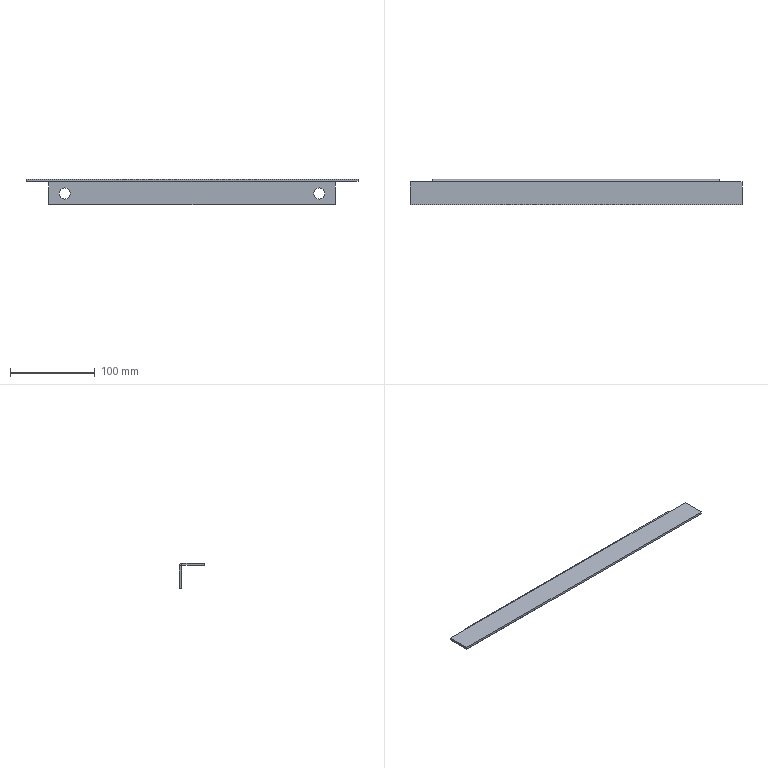Part | SolidWorks | features SMBaseFlange 2, Cut 1, EdgeFlange 1, FlatPattern 1, SheetMetal 1 | 1 solid | 20 faces | box 391 x 30 x 30 mm | volume 50792 mm3 | plane 14 | cylinder 6 | commonest cylinder face diameters 13 x4 1 x1 6 x1
STEP:
#1=CARTESIAN_POINT('',(150.,12.5,-23.25));
#2=VERTEX_POINT('',#1);
#3=CARTESIAN_POINT('',(150.,12.5,-10.25));
#4=VERTEX_POINT('',#3);
#5=CARTESIAN_POINT('',(150.,12.5,-16.75));
#6=DIRECTION('',(0.,1.,0.));
#7=DIRECTION('',(0.,0.,1.));
#8=AXIS2_PLACEMENT_3D('',#5,#6,#7);
#9=CIRCLE('',#8,6.5);
#10=EDGE_CURVE('',#2,#4,#9,.T.);
#11=ORIENTED_EDGE('',*,*,#10,.F.);
#12=CARTESIAN_POINT('',(150.,15.,-23.25));
#13=VERTEX_POINT('',#12);
#14=CARTESIAN_POINT('',(150.,12.5,-23.25));
#15=DIRECTION('',(0.,1.,0.));
#16=VECTOR('',#15,1000.);
#17=LINE('',#14,#16);
#18=EDGE_CURVE('',#2,#13,#17,.T.);
#19=ORIENTED_EDGE('',*,*,#18,.T.);
#20=CARTESIAN_POINT('',(150.,15.,-10.25));
#21=VERTEX_POINT('',#20);
#22=CARTESIAN_POINT('',(150.,15.,-16.75));
#23=DIRECTION('',(0.,1.,0.));
#24=DIRECTION('',(0.,0.,1.));
#25=AXIS2_PLACEMENT_3D('',#22,#23,#24);
#26=CIRCLE('',#25,6.5);
#27=EDGE_CURVE('',#13,#21,#26,.T.);
#28=ORIENTED_EDGE('',*,*,#27,.T.);
#29=CARTESIAN_POINT('',(150.,12.5,-10.25));
#30=DIRECTION('',(0.,1.,0.));
#31=VECTOR('',#30,1000.);
#32=LINE('',#29,#31);
#33=EDGE_CURVE('',#4,#21,#32,.T.);
#34=ORIENTED_EDGE('',*,*,#33,.F.);
#35=EDGE_LOOP('',(#11,#19,#28,#34));
#36=FACE_OUTER_BOUND('',#35,.T.);
#37=CARTESIAN_POINT('',(150.,12.5,-16.75));
#38=DIRECTION('',(0.,1.,0.));
#39=DIRECTION('',(0.,0.,1.));
#40=AXIS2_PLACEMENT_3D('',#37,#38,#39);
#41=CYLINDRICAL_SURFACE('',#40,6.5);
#42=ADVANCED_FACE('',(#36),#41,.F.);
#43=CARTESIAN_POINT('',(-150.,12.5,-23.25));
#44=VERTEX_POINT('',#43);
#45=CARTESIAN_POINT('',(-150.,12.5,-10.25));
#46=VERTEX_POINT('',#45);
#47=CARTESIAN_POINT('',(-150.,12.5,-16.75));
#48=DIRECTION('',(0.,1.,0.));
#49=DIRECTION('',(0.,0.,1.));
#50=AXIS2_PLACEMENT_3D('',#47,#48,#49);
#51=CIRCLE('',#50,6.5);
#52=EDGE_CURVE('',#44,#46,#51,.T.);
#53=ORIENTED_EDGE('',*,*,#52,.F.);
#54=CARTESIAN_POINT('',(-150.,15.,-23.25));
#55=VERTEX_POINT('',#54);
#56=CARTESIAN_POINT('',(-150.,12.5,-23.25));
#57=DIRECTION('',(0.,1.,0.));
#58=VECTOR('',#57,1000.);
#59=LINE('',#56,#58);
#60=EDGE_CURVE('',#44,#55,#59,.T.);
#61=ORIENTED_EDGE('',*,*,#60,.T.);
#62=CARTESIAN_POINT('',(-150.,15.,-10.25));
#63=VERTEX_POINT('',#62);
#64=CARTESIAN_POINT('',(-150.,15.,-16.75));
#65=DIRECTION('',(0.,1.,0.));
#66=DIRECTION('',(0.,0.,1.));
#67=AXIS2_PLACEMENT_3D('',#64,#65,#66);
#68=CIRCLE('',#67,6.5);
#69=EDGE_CURVE('',#55,#63,#68,.T.);
#70=ORIENTED_EDGE('',*,*,#69,.T.);
#71=CARTESIAN_POINT('',(-150.,12.5,-10.25));
#72=DIRECTION('',(0.,1.,0.));
#73=VECTOR('',#72,1000.);
#74=LINE('',#71,#73);
#75=EDGE_CURVE('',#46,#63,#74,.T.);
#76=ORIENTED_EDGE('',*,*,#75,.F.);
#77=EDGE_LOOP('',(#53,#61,#70,#76));
#78=FACE_OUTER_BOUND('',#77,.T.);
#79=CARTESIAN_POINT('',(-150.,12.5,-16.75));
#80=DIRECTION('',(0.,1.,0.));
#81=DIRECTION('',(0.,0.,1.));
#82=AXIS2_PLACEMENT_3D('',#79,#80,#81);
#83=CYLINDRICAL_SURFACE('',#82,6.5);
#84=ADVANCED_FACE('',(#78),#83,.F.);
#85=CARTESIAN_POINT('',(168.5,12.,-2.5));
#86=VERTEX_POINT('',#85);
#87=CARTESIAN_POINT('',(-168.5,12.,-2.5));
#88=VERTEX_POINT('',#87);
#89=CARTESIAN_POINT('',(168.5,12.,-2.5));
#90=DIRECTION('',(-1.,0.,0.));
#91=VECTOR('',#90,1000.);
#92=LINE('',#89,#91);
#93=EDGE_CURVE('',#86,#88,#92,.T.);
#94=ORIENTED_EDGE('',*,*,#93,.F.);
#95=CARTESIAN_POINT('',(195.5,12.,-2.5));
#96=VERTEX_POINT('',#95);
#97=CARTESIAN_POINT('',(168.5,12.,-2.5));
#98=DIRECTION('',(-1.,0.,0.));
#99=VECTOR('',#98,1000.);
#100=LINE('',#97,#99);
#101=EDGE_CURVE('',#96,#86,#100,.T.);
#102=ORIENTED_EDGE('',*,*,#101,.F.);
#103=CARTESIAN_POINT('',(195.5,-15.,-2.5));
#104=VERTEX_POINT('',#103);
#105=CARTESIAN_POINT('',(195.5,-15.,-2.5));
#106=DIRECTION('',(0.,1.,0.));
#107=VECTOR('',#106,1000.);
#108=LINE('',#105,#107);
#109=EDGE_CURVE('',#104,#96,#108,.T.);
#110=ORIENTED_EDGE('',*,*,#109,.F.);
#111=CARTESIAN_POINT('',(-195.5,-15.,-2.5));
#112=VERTEX_POINT('',#111);
#113=CARTESIAN_POINT('',(-168.5,-15.,-2.5));
#114=DIRECTION('',(1.,0.,0.));
#115=VECTOR('',#114,1000.);
#116=LINE('',#113,#115);
#117=EDGE_CURVE('',#112,#104,#116,.T.);
#118=ORIENTED_EDGE('',*,*,#117,.F.);
#119=CARTESIAN_POINT('',(-195.5,12.,-2.5));
#120=VERTEX_POINT('',#119);
#121=CARTESIAN_POINT('',(-195.5,-15.,-2.5));
#122=DIRECTION('',(0.,-1.,0.));
#123=VECTOR('',#122,1000.);
#124=LINE('',#121,#123);
#125=EDGE_CURVE('',#120,#112,#124,.T.);
#126=ORIENTED_EDGE('',*,*,#125,.F.);
#127=CARTESIAN_POINT('',(-168.5,12.,-2.5));
#128=DIRECTION('',(-1.,0.,0.));
#129=VECTOR('',#128,1000.);
#130=LINE('',#127,#129);
#131=EDGE_CURVE('',#88,#120,#130,.T.);
#132=ORIENTED_EDGE('',*,*,#131,.F.);
#133=EDGE_LOOP('',(#94,#102,#110,#118,#126,#132));
#134=FACE_OUTER_BOUND('',#133,.T.);
#135=CARTESIAN_POINT('',(0.,0.,-2.5));
#136=DIRECTION('',(0.,0.,1.));
#137=DIRECTION('',(1.,0.,0.));
#138=AXIS2_PLACEMENT_3D('',#135,#136,#137);
#139=PLANE('',#138);
#140=ADVANCED_FACE('',(#134),#139,.F.);
#141=CARTESIAN_POINT('',(-195.5,-15.,0.));
#142=VERTEX_POINT('',#141);
#143=CARTESIAN_POINT('',(195.5,-15.,0.));
#144=VERTEX_POINT('',#143);
#145=CARTESIAN_POINT('',(-168.5,-15.,0.));
#146=DIRECTION('',(1.,0.,0.));
#147=VECTOR('',#146,1000.);
#148=LINE('',#145,#147);
#149=EDGE_CURVE('',#142,#144,#148,.T.);
#150=ORIENTED_EDGE('',*,*,#149,.T.);
#151=CARTESIAN_POINT('',(195.5,12.,0.));
#152=VERTEX_POINT('',#151);
#153=CARTESIAN_POINT('',(195.5,-15.,0.));
#154=DIRECTION('',(0.,1.,0.));
#155=VECTOR('',#154,1000.);
#156=LINE('',#153,#155);
#157=EDGE_CURVE('',#144,#152,#156,.T.);
#158=ORIENTED_EDGE('',*,*,#157,.T.);
#159=CARTESIAN_POINT('',(168.5,12.,0.));
#160=VERTEX_POINT('',#159);
#161=CARTESIAN_POINT('',(168.5,12.,0.));
#162=DIRECTION('',(-1.,0.,0.));
#163=VECTOR('',#162,1000.);
#164=LINE('',#161,#163);
#165=EDGE_CURVE('',#152,#160,#164,.T.);
#166=ORIENTED_EDGE('',*,*,#165,.T.);
#167=CARTESIAN_POINT('',(-168.5,12.,0.));
#168=VERTEX_POINT('',#167);
#169=CARTESIAN_POINT('',(168.5,12.,0.));
#170=DIRECTION('',(-1.,0.,0.));
#171=VECTOR('',#170,1000.);
#172=LINE('',#169,#171);
#173=EDGE_CURVE('',#160,#168,#172,.T.);
#174=ORIENTED_EDGE('',*,*,#173,.T.);
#175=CARTESIAN_POINT('',(-195.5,12.,0.));
#176=VERTEX_POINT('',#175);
#177=CARTESIAN_POINT('',(-168.5,12.,0.));
#178=DIRECTION('',(-1.,0.,0.));
#179=VECTOR('',#178,1000.);
#180=LINE('',#177,#179);
#181=EDGE_CURVE('',#168,#176,#180,.T.);
#182=ORIENTED_EDGE('',*,*,#181,.T.);
#183=CARTESIAN_POINT('',(-195.5,-15.,0.));
#184=DIRECTION('',(0.,-1.,0.));
#185=VECTOR('',#184,1000.);
#186=LINE('',#183,#185);
#187=EDGE_CURVE('',#176,#142,#186,.T.);
#188=ORIENTED_EDGE('',*,*,#187,.T.);
#189=EDGE_LOOP('',(#150,#158,#166,#174,#182,#188));
#190=FACE_OUTER_BOUND('',#189,.T.);
#191=CARTESIAN_POINT('',(0.,0.,0.));
#192=DIRECTION('',(0.,0.,1.));
#193=DIRECTION('',(1.,0.,0.));
#194=AXIS2_PLACEMENT_3D('',#191,#192,#193);
#195=PLANE('',#194);
#196=ADVANCED_FACE('',(#190),#195,.T.);
#197=ORIENTED_EDGE('',*,*,#149,.F.);
#198=CARTESIAN_POINT('',(-195.5,-15.,-2.5));
#199=DIRECTION('',(0.,0.,1.));
#200=VECTOR('',#199,1000.);
#201=LINE('',#198,#200);
#202=EDGE_CURVE('',#112,#142,#201,.T.);
#203=ORIENTED_EDGE('',*,*,#202,.F.);
#204=ORIENTED_EDGE('',*,*,#117,.T.);
#205=CARTESIAN_POINT('',(195.5,-15.,-2.5));
#206=DIRECTION('',(0.,0.,1.));
#207=VECTOR('',#206,1000.);
#208=LINE('',#205,#207);
#209=EDGE_CURVE('',#104,#144,#208,.T.);
#210=ORIENTED_EDGE('',*,*,#209,.T.);
#211=EDGE_LOOP('',(#197,#203,#204,#210));
#212=FACE_OUTER_BOUND('',#211,.T.);
#213=CARTESIAN_POINT('',(-168.5,-15.,-2.5));
#214=DIRECTION('',(0.,-1.,0.));
#215=DIRECTION('',(0.,0.,-1.));
#216=AXIS2_PLACEMENT_3D('',#213,#214,#215);
#217=PLANE('',#216);
#218=ADVANCED_FACE('',(#212),#217,.T.);
#219=CARTESIAN_POINT('',(-168.5,12.5,-3.));
#220=VERTEX_POINT('',#219);
#221=CARTESIAN_POINT('',(-168.5,15.,-3.));
#222=VERTEX_POINT('',#221);
#223=CARTESIAN_POINT('',(-168.5,15.,-3.));
#224=DIRECTION('',(0.,1.,0.));
#225=VECTOR('',#224,1000.);
#226=LINE('',#223,#225);
#227=EDGE_CURVE('',#220,#222,#226,.T.);
#228=ORIENTED_EDGE('',*,*,#227,.F.);
#229=CARTESIAN_POINT('',(-168.5,12.,-3.));
#230=DIRECTION('',(-1.,0.,0.));
#231=DIRECTION('',(0.,0.,-1.));
#232=AXIS2_PLACEMENT_3D('',#229,#230,#231);
#233=CIRCLE('',#232,0.5);
#234=EDGE_CURVE('',#88,#220,#233,.T.);
#235=ORIENTED_EDGE('',*,*,#234,.F.);
#236=CARTESIAN_POINT('',(-168.5,12.,-2.5));
#237=DIRECTION('',(0.,0.,1.));
#238=VECTOR('',#237,1000.);
#239=LINE('',#236,#238);
#240=EDGE_CURVE('',#88,#168,#239,.T.);
#241=ORIENTED_EDGE('',*,*,#240,.T.);
#242=CARTESIAN_POINT('',(-168.5,12.,-3.));
#243=DIRECTION('',(-1.,0.,0.));
#244=DIRECTION('',(0.,0.,-1.));
#245=AXIS2_PLACEMENT_3D('',#242,#243,#244);
#246=CIRCLE('',#245,3.);
#247=EDGE_CURVE('',#168,#222,#246,.T.);
#248=ORIENTED_EDGE('',*,*,#247,.T.);
#249=EDGE_LOOP('',(#228,#235,#241,#248));
#250=FACE_OUTER_BOUND('',#249,.T.);
#251=CARTESIAN_POINT('',(-168.5,12.,-3.));
#252=DIRECTION('',(-1.,0.,0.));
#253=DIRECTION('',(0.,0.,1.));
#254=AXIS2_PLACEMENT_3D('',#251,#252,#253);
#255=PLANE('',#254);
#256=ADVANCED_FACE('',(#250),#255,.T.);
#257=CARTESIAN_POINT('',(168.5,12.5,-3.));
#258=VERTEX_POINT('',#257);
#259=CARTESIAN_POINT('',(168.5,12.,-3.));
#260=DIRECTION('',(1.,0.,0.));
#261=DIRECTION('',(0.,0.,-1.));
#262=AXIS2_PLACEMENT_3D('',#259,#260,#261);
#263=CIRCLE('',#262,0.5);
#264=EDGE_CURVE('',#258,#86,#263,.T.);
#265=ORIENTED_EDGE('',*,*,#264,.F.);
#266=CARTESIAN_POINT('',(168.5,15.,-3.));
#267=VERTEX_POINT('',#266);
#268=CARTESIAN_POINT('',(168.5,12.5,-3.));
#269=DIRECTION('',(0.,1.,0.));
#270=VECTOR('',#269,1000.);
#271=LINE('',#268,#270);
#272=EDGE_CURVE('',#258,#267,#271,.T.);
#273=ORIENTED_EDGE('',*,*,#272,.T.);
#274=CARTESIAN_POINT('',(168.5,12.,-3.));
#275=DIRECTION('',(1.,0.,0.));
#276=DIRECTION('',(0.,0.,-1.));
#277=AXIS2_PLACEMENT_3D('',#274,#275,#276);
#278=CIRCLE('',#277,3.);
#279=EDGE_CURVE('',#267,#160,#278,.T.);
#280=ORIENTED_EDGE('',*,*,#279,.T.);
#281=CARTESIAN_POINT('',(168.5,12.,-2.5));
#282=DIRECTION('',(0.,0.,1.));
#283=VECTOR('',#282,1000.);
#284=LINE('',#281,#283);
#285=EDGE_CURVE('',#86,#160,#284,.T.);
#286=ORIENTED_EDGE('',*,*,#285,.F.);
#287=EDGE_LOOP('',(#265,#273,#280,#286));
#288=FACE_OUTER_BOUND('',#287,.T.);
#289=CARTESIAN_POINT('',(168.5,12.,-3.));
#290=DIRECTION('',(-1.,0.,0.));
#291=DIRECTION('',(0.,0.,1.));
#292=AXIS2_PLACEMENT_3D('',#289,#290,#291);
#293=PLANE('',#292);
#294=ADVANCED_FACE('',(#288),#293,.F.);
#295=ORIENTED_EDGE('',*,*,#173,.F.);
#296=ORIENTED_EDGE('',*,*,#279,.F.);
#297=CARTESIAN_POINT('',(0.,15.,-3.));
#298=DIRECTION('',(1.,0.,0.));
#299=VECTOR('',#298,1000.);
#300=LINE('',#297,#299);
#301=EDGE_CURVE('',#222,#267,#300,.T.);
#302=ORIENTED_EDGE('',*,*,#301,.F.);
#303=ORIENTED_EDGE('',*,*,#247,.F.);
#304=EDGE_LOOP('',(#295,#296,#302,#303));
#305=FACE_OUTER_BOUND('',#304,.T.);
#306=CARTESIAN_POINT('',(168.5,12.,-3.));
#307=DIRECTION('',(1.,0.,0.));
#308=DIRECTION('',(0.,1.,0.));
#309=AXIS2_PLACEMENT_3D('',#306,#307,#308);
#310=CYLINDRICAL_SURFACE('',#309,3.);
#311=ADVANCED_FACE('',(#305),#310,.T.);
#312=ORIENTED_EDGE('',*,*,#93,.T.);
#313=ORIENTED_EDGE('',*,*,#234,.T.);
#314=CARTESIAN_POINT('',(-168.5,12.5,-3.));
#315=DIRECTION('',(1.,0.,0.));
#316=VECTOR('',#315,1000.);
#317=LINE('',#314,#316);
#318=EDGE_CURVE('',#220,#258,#317,.T.);
#319=ORIENTED_EDGE('',*,*,#318,.T.);
#320=ORIENTED_EDGE('',*,*,#264,.T.);
#321=EDGE_LOOP('',(#312,#313,#319,#320));
#322=FACE_OUTER_BOUND('',#321,.T.);
#323=CARTESIAN_POINT('',(168.5,12.,-3.));
#324=DIRECTION('',(1.,0.,0.));
#325=DIRECTION('',(0.,1.,0.));
#326=AXIS2_PLACEMENT_3D('',#323,#324,#325);
#327=CYLINDRICAL_SURFACE('',#326,0.5);
#328=ADVANCED_FACE('',(#322),#327,.F.);
#329=CARTESIAN_POINT('',(168.5,15.,-30.));
#330=VERTEX_POINT('',#329);
#331=CARTESIAN_POINT('',(168.5,15.,-2.5));
#332=DIRECTION('',(0.,0.,1.));
#333=VECTOR('',#332,1000.);
#334=LINE('',#331,#333);
#335=EDGE_CURVE('',#330,#267,#334,.T.);
#336=ORIENTED_EDGE('',*,*,#335,.T.);
#337=ORIENTED_EDGE('',*,*,#272,.F.);
#338=CARTESIAN_POINT('',(168.5,12.5,-30.));
#339=VERTEX_POINT('',#338);
#340=CARTESIAN_POINT('',(168.5,12.5,0.));
#341=DIRECTION('',(0.,0.,1.));
#342=VECTOR('',#341,1000.);
#343=LINE('',#340,#342);
#344=EDGE_CURVE('',#339,#258,#343,.T.);
#345=ORIENTED_EDGE('',*,*,#344,.F.);
#346=CARTESIAN_POINT('',(168.5,15.,-30.));
#347=DIRECTION('',(0.,-1.,0.));
#348=VECTOR('',#347,1000.);
#349=LINE('',#346,#348);
#350=EDGE_CURVE('',#330,#339,#349,.T.);
#351=ORIENTED_EDGE('',*,*,#350,.F.);
#352=EDGE_LOOP('',(#336,#337,#345,#351));
#353=FACE_OUTER_BOUND('',#352,.T.);
#354=CARTESIAN_POINT('',(168.5,15.,-2.5));
#355=DIRECTION('',(1.,0.,0.));
#356=DIRECTION('',(0.,0.,-1.));
#357=AXIS2_PLACEMENT_3D('',#354,#355,#356);
#358=PLANE('',#357);
#359=ADVANCED_FACE('',(#353),#358,.T.);
#360=CARTESIAN_POINT('',(-168.5,12.5,-30.));
#361=VERTEX_POINT('',#360);
#362=CARTESIAN_POINT('',(-168.5,12.5,0.));
#363=DIRECTION('',(0.,0.,-1.));
#364=VECTOR('',#363,1000.);
#365=LINE('',#362,#364);
#366=EDGE_CURVE('',#220,#361,#365,.T.);
#367=ORIENTED_EDGE('',*,*,#366,.F.);
#368=ORIENTED_EDGE('',*,*,#227,.T.);
#369=CARTESIAN_POINT('',(-168.5,15.,-30.));
#370=VERTEX_POINT('',#369);
#371=CARTESIAN_POINT('',(-168.5,15.,-30.));
#372=DIRECTION('',(0.,0.,-1.));
#373=VECTOR('',#372,1000.);
#374=LINE('',#371,#373);
#375=EDGE_CURVE('',#222,#370,#374,.T.);
#376=ORIENTED_EDGE('',*,*,#375,.T.);
#377=CARTESIAN_POINT('',(-168.5,15.,-30.));
#378=DIRECTION('',(0.,-1.,0.));
#379=VECTOR('',#378,1000.);
#380=LINE('',#377,#379);
#381=EDGE_CURVE('',#370,#361,#380,.T.);
#382=ORIENTED_EDGE('',*,*,#381,.T.);
#383=EDGE_LOOP('',(#367,#368,#376,#382));
#384=FACE_OUTER_BOUND('',#383,.T.);
#385=CARTESIAN_POINT('',(-168.5,15.,-30.));
#386=DIRECTION('',(-1.,0.,0.));
#387=DIRECTION('',(0.,0.,1.));
#388=AXIS2_PLACEMENT_3D('',#385,#386,#387);
#389=PLANE('',#388);
#390=ADVANCED_FACE('',(#384),#389,.T.);
#391=CARTESIAN_POINT('',(150.,15.,-16.75));
#392=DIRECTION('',(0.,1.,0.));
#393=DIRECTION('',(0.,0.,1.));
#394=AXIS2_PLACEMENT_3D('',#391,#392,#393);
#395=CIRCLE('',#394,6.5);
#396=EDGE_CURVE('',#21,#13,#395,.T.);
#397=ORIENTED_EDGE('',*,*,#396,.F.);
#398=ORIENTED_EDGE('',*,*,#27,.F.);
#399=EDGE_LOOP('',(#397,#398));
#400=FACE_BOUND('',#399,.T.);
#401=CARTESIAN_POINT('',(-150.,15.,-16.75));
#402=DIRECTION('',(0.,1.,0.));
#403=DIRECTION('',(0.,0.,1.));
#404=AXIS2_PLACEMENT_3D('',#401,#402,#403);
#405=CIRCLE('',#404,6.5);
#406=EDGE_CURVE('',#63,#55,#405,.T.);
#407=ORIENTED_EDGE('',*,*,#406,.F.);
#408=ORIENTED_EDGE('',*,*,#69,.F.);
#409=EDGE_LOOP('',(#407,#408));
#410=FACE_BOUND('',#409,.T.);
#411=ORIENTED_EDGE('',*,*,#375,.F.);
#412=ORIENTED_EDGE('',*,*,#301,.T.);
#413=ORIENTED_EDGE('',*,*,#335,.F.);
#414=CARTESIAN_POINT('',(168.5,15.,-30.));
#415=DIRECTION('',(1.,0.,0.));
#416=VECTOR('',#415,1000.);
#417=LINE('',#414,#416);
#418=EDGE_CURVE('',#370,#330,#417,.T.);
#419=ORIENTED_EDGE('',*,*,#418,.F.);
#420=EDGE_LOOP('',(#411,#412,#413,#419));
#421=FACE_OUTER_BOUND('',#420,.T.);
#422=CARTESIAN_POINT('',(0.,15.,0.));
#423=DIRECTION('',(0.,1.,0.));
#424=DIRECTION('',(0.,0.,1.));
#425=AXIS2_PLACEMENT_3D('',#422,#423,#424);
#426=PLANE('',#425);
#427=ADVANCED_FACE('',(#400,#410,#421),#426,.T.);
#428=CARTESIAN_POINT('',(150.,12.5,-16.75));
#429=DIRECTION('',(0.,1.,0.));
#430=DIRECTION('',(0.,0.,1.));
#431=AXIS2_PLACEMENT_3D('',#428,#429,#430);
#432=CIRCLE('',#431,6.5);
#433=EDGE_CURVE('',#4,#2,#432,.T.);
#434=ORIENTED_EDGE('',*,*,#433,.T.);
#435=ORIENTED_EDGE('',*,*,#10,.T.);
#436=EDGE_LOOP('',(#434,#435));
#437=FACE_BOUND('',#436,.T.);
#438=CARTESIAN_POINT('',(-150.,12.5,-16.75));
#439=DIRECTION('',(0.,1.,0.));
#440=DIRECTION('',(0.,0.,1.));
#441=AXIS2_PLACEMENT_3D('',#438,#439,#440);
#442=CIRCLE('',#441,6.5);
#443=EDGE_CURVE('',#46,#44,#442,.T.);
#444=ORIENTED_EDGE('',*,*,#443,.T.);
#445=ORIENTED_EDGE('',*,*,#52,.T.);
#446=EDGE_LOOP('',(#444,#445));
#447=FACE_BOUND('',#446,.T.);
#448=ORIENTED_EDGE('',*,*,#318,.F.);
#449=ORIENTED_EDGE('',*,*,#366,.T.);
#450=CARTESIAN_POINT('',(0.,12.5,-30.));
#451=DIRECTION('',(1.,0.,0.));
#452=VECTOR('',#451,1000.);
#453=LINE('',#450,#452);
#454=EDGE_CURVE('',#361,#339,#453,.T.);
#455=ORIENTED_EDGE('',*,*,#454,.T.);
#456=ORIENTED_EDGE('',*,*,#344,.T.);
#457=EDGE_LOOP('',(#448,#449,#455,#456));
#458=FACE_OUTER_BOUND('',#457,.T.);
#459=CARTESIAN_POINT('',(0.,12.5,0.));
#460=DIRECTION('',(0.,1.,0.));
#461=DIRECTION('',(0.,0.,1.));
#462=AXIS2_PLACEMENT_3D('',#459,#460,#461);
#463=PLANE('',#462);
#464=ADVANCED_FACE('',(#437,#447,#458),#463,.F.);
#465=ORIENTED_EDGE('',*,*,#454,.F.);
#466=ORIENTED_EDGE('',*,*,#381,.F.);
#467=ORIENTED_EDGE('',*,*,#418,.T.);
#468=ORIENTED_EDGE('',*,*,#350,.T.);
#469=EDGE_LOOP('',(#465,#466,#467,#468));
#470=FACE_OUTER_BOUND('',#469,.T.);
#471=CARTESIAN_POINT('',(168.5,15.,-30.));
#472=DIRECTION('',(0.,0.,-1.));
#473=DIRECTION('',(0.,1.,0.));
#474=AXIS2_PLACEMENT_3D('',#471,#472,#473);
#475=PLANE('',#474);
#476=ADVANCED_FACE('',(#470),#475,.T.);
#477=ORIENTED_EDGE('',*,*,#187,.F.);
#478=CARTESIAN_POINT('',(-195.5,12.,-2.5));
#479=DIRECTION('',(0.,0.,1.));
#480=VECTOR('',#479,1000.);
#481=LINE('',#478,#480);
#482=EDGE_CURVE('',#120,#176,#481,.T.);
#483=ORIENTED_EDGE('',*,*,#482,.F.);
#484=ORIENTED_EDGE('',*,*,#125,.T.);
#485=ORIENTED_EDGE('',*,*,#202,.T.);
#486=EDGE_LOOP('',(#477,#483,#484,#485));
#487=FACE_OUTER_BOUND('',#486,.T.);
#488=CARTESIAN_POINT('',(-195.5,-15.,-2.5));
#489=DIRECTION('',(-1.,0.,0.));
#490=DIRECTION('',(0.,0.,1.));
#491=AXIS2_PLACEMENT_3D('',#488,#489,#490);
#492=PLANE('',#491);
#493=ADVANCED_FACE('',(#487),#492,.T.);
#494=ORIENTED_EDGE('',*,*,#181,.F.);
#495=ORIENTED_EDGE('',*,*,#240,.F.);
#496=ORIENTED_EDGE('',*,*,#131,.T.);
#497=ORIENTED_EDGE('',*,*,#482,.T.);
#498=EDGE_LOOP('',(#494,#495,#496,#497));
#499=FACE_OUTER_BOUND('',#498,.T.);
#500=CARTESIAN_POINT('',(-168.5,12.,-2.5));
#501=DIRECTION('',(0.,1.,0.));
#502=DIRECTION('',(-1.,0.,0.));
#503=AXIS2_PLACEMENT_3D('',#500,#501,#502);
#504=PLANE('',#503);
#505=ADVANCED_FACE('',(#499),#504,.T.);
#506=ORIENTED_EDGE('',*,*,#165,.F.);
#507=CARTESIAN_POINT('',(195.5,12.,-2.5));
#508=DIRECTION('',(0.,0.,1.));
#509=VECTOR('',#508,1000.);
#510=LINE('',#507,#509);
#511=EDGE_CURVE('',#96,#152,#510,.T.);
#512=ORIENTED_EDGE('',*,*,#511,.F.);
#513=ORIENTED_EDGE('',*,*,#101,.T.);
#514=ORIENTED_EDGE('',*,*,#285,.T.);
#515=EDGE_LOOP('',(#506,#512,#513,#514));
#516=FACE_OUTER_BOUND('',#515,.T.);
#517=CARTESIAN_POINT('',(168.5,12.,-2.5));
#518=DIRECTION('',(0.,1.,0.));
#519=DIRECTION('',(-1.,0.,0.));
#520=AXIS2_PLACEMENT_3D('',#517,#518,#519);
#521=PLANE('',#520);
#522=ADVANCED_FACE('',(#516),#521,.T.);
#523=ORIENTED_EDGE('',*,*,#157,.F.);
#524=ORIENTED_EDGE('',*,*,#209,.F.);
#525=ORIENTED_EDGE('',*,*,#109,.T.);
#526=ORIENTED_EDGE('',*,*,#511,.T.);
#527=EDGE_LOOP('',(#523,#524,#525,#526));
#528=FACE_OUTER_BOUND('',#527,.T.);
#529=CARTESIAN_POINT('',(195.5,-15.,-2.5));
#530=DIRECTION('',(1.,0.,0.));
#531=DIRECTION('',(0.,0.,-1.));
#532=AXIS2_PLACEMENT_3D('',#529,#530,#531);
#533=PLANE('',#532);
#534=ADVANCED_FACE('',(#528),#533,.T.);
#535=ORIENTED_EDGE('',*,*,#60,.F.);
#536=ORIENTED_EDGE('',*,*,#443,.F.);
#537=ORIENTED_EDGE('',*,*,#75,.T.);
#538=ORIENTED_EDGE('',*,*,#406,.T.);
#539=EDGE_LOOP('',(#535,#536,#537,#538));
#540=FACE_OUTER_BOUND('',#539,.T.);
#541=CARTESIAN_POINT('',(-150.,12.5,-16.75));
#542=DIRECTION('',(0.,1.,0.));
#543=DIRECTION('',(0.,0.,1.));
#544=AXIS2_PLACEMENT_3D('',#541,#542,#543);
#545=CYLINDRICAL_SURFACE('',#544,6.5);
#546=ADVANCED_FACE('',(#540),#545,.F.);
#547=ORIENTED_EDGE('',*,*,#18,.F.);
#548=ORIENTED_EDGE('',*,*,#433,.F.);
#549=ORIENTED_EDGE('',*,*,#33,.T.);
#550=ORIENTED_EDGE('',*,*,#396,.T.);
#551=EDGE_LOOP('',(#547,#548,#549,#550));
#552=FACE_OUTER_BOUND('',#551,.T.);
#553=CARTESIAN_POINT('',(150.,12.5,-16.75));
#554=DIRECTION('',(0.,1.,0.));
#555=DIRECTION('',(0.,0.,1.));
#556=AXIS2_PLACEMENT_3D('',#553,#554,#555);
#557=CYLINDRICAL_SURFACE('',#556,6.5);
#558=ADVANCED_FACE('',(#552),#557,.F.);
#559=CLOSED_SHELL('',(#42,#84,#140,#196,#218,#256,#294,#311,#328,#359,#390,#427,#464,#476,#493,#505,#522,#534,#546,#558));
#560=MANIFOLD_SOLID_BREP('',#559);
#561=CARTESIAN_POINT('',(0.,0.,0.));
#562=DIRECTION('',(0.,0.,1.));
#563=DIRECTION('',(1.,0.,0.));
#564=AXIS2_PLACEMENT_3D('',#561,#562,#563);
#565=(LENGTH_UNIT()NAMED_UNIT(*)SI_UNIT(.MILLI.,.METRE.));
#566=UNCERTAINTY_MEASURE_WITH_UNIT(LENGTH_MEASURE(0.00001),#565,'','');
#567=(NAMED_UNIT(*)PLANE_ANGLE_UNIT()SI_UNIT($,.RADIAN.));
#568=(NAMED_UNIT(*)SI_UNIT($,.STERADIAN.)SOLID_ANGLE_UNIT());
#569=(GEOMETRIC_REPRESENTATION_CONTEXT(3)GLOBAL_UNCERTAINTY_ASSIGNED_CONTEXT((#566))GLOBAL_UNIT_ASSIGNED_CONTEXT((#565,#567,#568))REPRESENTATION_CONTEXT('',''));
#570=ADVANCED_BREP_SHAPE_REPRESENTATION('',(#560,#564),#569);